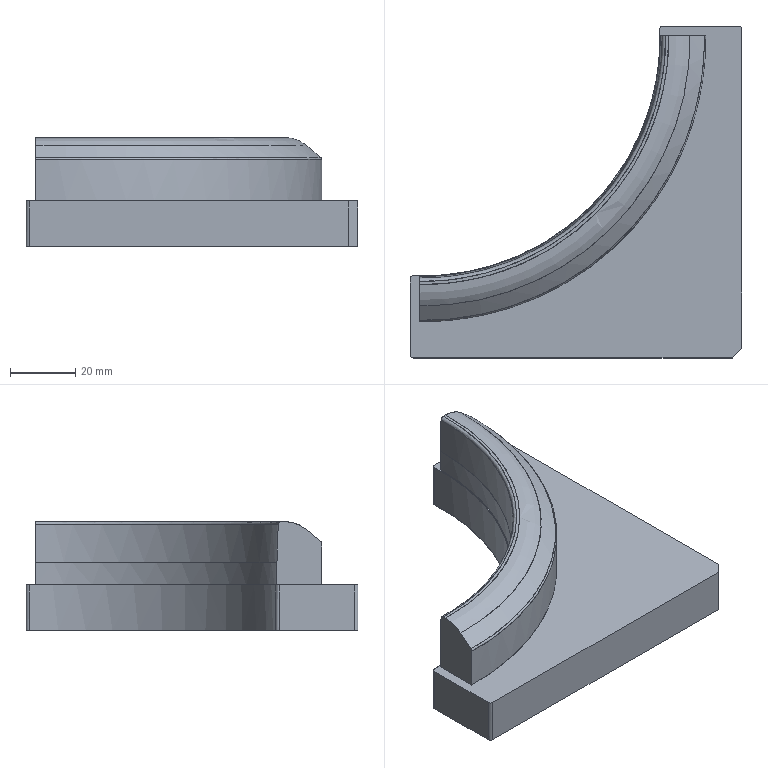CAM job | PowerMill | 3-axis milling, other | part box 102 x 102 x 33.478 mm
Tools:
number,name,type,diameter,tip_radius,length,cutting_length,overhang,flutes,holder,toolpaths_using
1,D10C_1_1_1,end_mill,10.0,0.0,60.0,,33.92,1,D42L35,8
3,D10_1_1_1,end_mill,10.0,0.0,60.0,,33.64,1,D42L35,8
7,R2_1_1_1,ball_nosed,4.0,2.0,30.0,,14.84,1,D42L35,2
13,Text_D4_1_1,taper_spherical,4.0,0.3,60.0,,19.72,1,D42L35,2
7,R2_2_1_1,ball_nosed,4.0,2.0,30.0,,14.64,1,D42L35,2
Operations:
program,toolpath,strategy,tool,tool_number,tool_diameter,tip_radius,flutes,spindle_rpm,feed_cut,surface_speed_m_min_computed,feed_per_tooth_computed,tolerance,thickness,stepover,stepdown,cut_length,cut_time_min,total_time_min,workplane
21-A-1-F,精公开粗01-扫面平行-D10C,raster_area_clear,D10C_1_1_1,1,10.0,0.0,1.0,8000.0,10000.0,251.33,1.25,0.03,0.28,6.0,1.0,2586.32,0.259,0.2704,
21-A-1-F,精公开粗01-外形偏置-D10C,offset_area_clear,D10C_1_1_1,1,10.0,0.0,1.0,8000.0,10000.0,251.33,1.25,0.03,0.28,6.0,1.0,113986.48,11.399,11.525,
21-A-1-F,精公开粗01-平行中光-D10C,raster,D10C_1_1_1,1,10.0,0.0,1.0,8000.0,10000.0,251.33,1.25,0.03,0.28,0.3,1.0,11154.302,1.115,1.15,
21-A-1-F,精公开粗01-基准台偏置-D10C,offset_area_clear,D10C_1_1_1,1,10.0,0.0,1.0,8000.0,10000.0,251.33,1.25,0.03,0.07,6.0,1.0,55714.673,5.572,5.638,
21-A-1-F,精公基准台01-平坦面平行-D10,raster_area_clear,D10_1_1_1,3,10.0,0.0,1.0,8500.0,600.0,267.04,0.0706,0.005,0.38,5.0,1.0,431.29,0.719,0.738,
21-A-1-F,精公基准台01-基准面偏置-D10,offset_area_clear,D10_1_1_1,3,10.0,0.0,1.0,8500.0,600.0,267.04,0.0706,0.005,0.38,5.0,1.0,1031.16,1.719,1.742,
21-A-1-F,精公基准台01-外形侧光-D10,profile_area_clear,D10_1_1_1,3,10.0,0.0,1.0,8500.0,600.0,267.04,0.0706,0.005,-0.07,0.08,1.0,627.892,1.046,1.08,
21-A-1-F,精公基准台01-基准台侧光-D10,profile_area_clear,D10_1_1_1,3,10.0,0.0,1.0,8500.0,600.0,267.04,0.0706,0.005,0.0,0.08,1.0,810.122,1.35,1.423,
21-A-1-F,精公精光01-平行-R2,raster,R2_1_1_1,7,4.0,2.0,1.0,18000.0,2000.0,226.19,0.1111,0.005,-0.075,0.05,1.0,54028.684,27.014,27.269,
21-A-1-F,精公精光02-等高-R2,constantz,R2_1_1_1,7,4.0,2.0,1.0,18000.0,2000.0,226.19,0.1111,0.005,-0.075,5.0,0.05,27409.087,13.704,13.965,
21-A-1-F,精公刻字01-刻字-Text_D4,pattern,Text_D4_1_1,13,4.0,0.3,1.0,15000.0,1000.0,188.5,0.0667,0.005,0.0,5.0,1.0,79.164,0.079,0.1053,
21-A-1-R,粗公开粗01-扫面平行-D10C,raster_area_clear,D10C_1_1_1,1,10.0,0.0,1.0,8000.0,10000.0,251.33,1.25,0.03,0.15,6.0,1.0,5165.6,0.517,0.5294,
21-A-1-R,粗公开粗01-外形偏置-D10C,offset_area_clear,D10C_1_1_1,1,10.0,0.0,1.0,8000.0,10000.0,251.33,1.25,0.03,0.15,6.0,1.0,113907.317,11.391,11.518,
21-A-1-R,粗公开粗01-平行中光-D10C,raster,D10C_1_1_1,1,10.0,0.0,1.0,8000.0,10000.0,251.33,1.25,0.03,0.15,0.3,1.0,10976.531,1.098,1.132,
21-A-1-R,粗公开粗01-基准台偏置-D10C,offset_area_clear,D10C_1_1_1,1,10.0,0.0,1.0,8000.0,10000.0,251.33,1.25,0.03,0.07,6.0,1.0,55714.673,5.572,5.638,
21-A-1-R,粗公基准台01-平坦面平行-D10,raster_area_clear,D10_1_1_1,3,10.0,0.0,1.0,8500.0,600.0,267.04,0.0706,0.01,0.25,5.0,1.0,402.187,0.67,0.6913,
21-A-1-R,粗公基准台01-基准面偏置-D10,offset_area_clear,D10_1_1_1,3,10.0,0.0,1.0,8500.0,600.0,267.04,0.0706,0.01,0.25,5.0,1.0,1028.179,1.714,1.736,
21-A-1-R,粗公基准台01-外形侧光-D10,profile_area_clear,D10_1_1_1,3,10.0,0.0,1.0,8500.0,600.0,267.04,0.0706,0.01,-0.2,0.08,1.0,626.254,1.044,1.077,
21-A-1-R,粗公基准台01-基准台侧光-D10,profile_area_clear,D10_1_1_1,3,10.0,0.0,1.0,8500.0,600.0,267.04,0.0706,0.01,0.0,0.08,1.0,810.094,1.35,1.423,
21-A-1-R,粗公精光01-平行-R2,raster,R2_2_1_1,7,4.0,2.0,1.0,18000.0,2000.0,226.19,0.1111,0.01,-0.205,0.06,1.0,44009.842,22.005,22.258,
21-A-1-R,粗公精光02-等高-R2,constantz,R2_2_1_1,7,4.0,2.0,1.0,18000.0,2000.0,226.19,0.1111,0.01,-0.205,5.0,0.06,22618.585,11.309,11.601,
21-A-1-R,粗公刻字01-刻字-Text_D4,pattern,Text_D4_1_1,13,4.0,0.3,1.0,15000.0,1000.0,188.5,0.0667,0.01,0.0,5.0,1.0,70.457,0.07,0.0952,